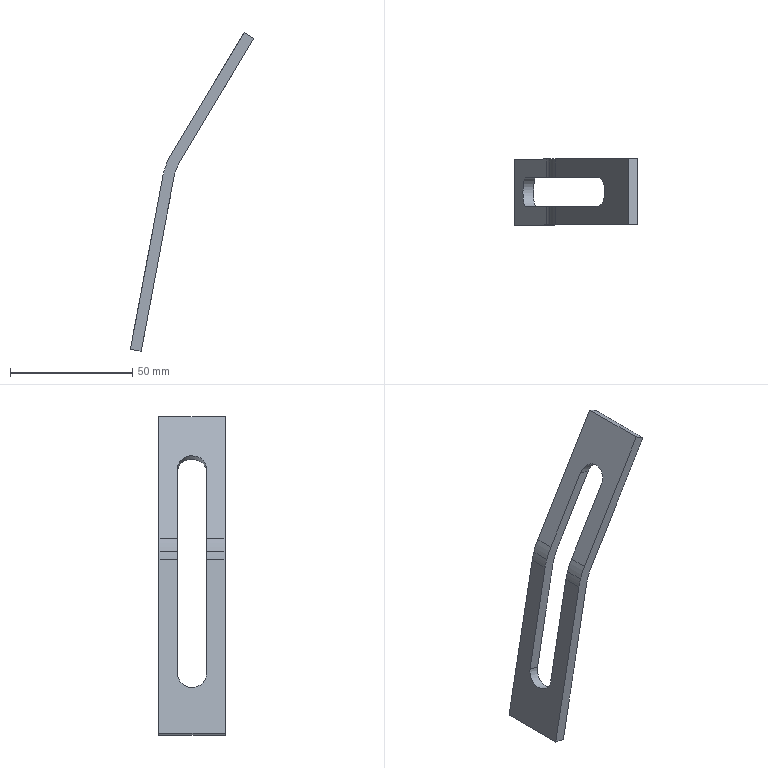Part | STEP file | 2026.6.15-Main Assembly图.sldasm-Part-201 | 1 solid | 20 faces | box 50.44 x 27 x 130.381 mm | volume 11515 mm3 | cylinder 10 | plane 10 | commonest cylinder face diameters 43.5 x4 52.5 x4 12 x2
STEP:
#1=CARTESIAN_POINT('',(-1667.232,1410.764,3344.403));
#2=VERTEX_POINT('',#1);
#3=CARTESIAN_POINT('',(-1667.232,1418.264,3344.403));
#4=VERTEX_POINT('',#3);
#5=CARTESIAN_POINT('',(-1667.232,1410.764,3344.403));
#6=DIRECTION('',(0.,1.,0.));
#7=VECTOR('',#6,1000.);
#8=LINE('',#5,#7);
#9=EDGE_CURVE('',#2,#4,#8,.T.);
#10=ORIENTED_EDGE('',*,*,#9,.F.);
#11=CARTESIAN_POINT('',(-1668.,1410.764,3341.468));
#12=VERTEX_POINT('',#11);
#13=CARTESIAN_POINT('',(-1646.625,1410.764,3337.444));
#14=DIRECTION('',(0.,1.,0.));
#15=DIRECTION('',(-0.9474,0.,0.3199));
#16=AXIS2_PLACEMENT_3D('',#13,#14,#15);
#17=CIRCLE('',#16,21.75);
#18=EDGE_CURVE('',#12,#2,#17,.T.);
#19=ORIENTED_EDGE('',*,*,#18,.F.);
#20=CARTESIAN_POINT('',(-1668.,1418.264,3341.468));
#21=VERTEX_POINT('',#20);
#22=CARTESIAN_POINT('',(-1668.,1410.764,3341.468));
#23=DIRECTION('',(0.,-1.,0.));
#24=VECTOR('',#23,1000.);
#25=LINE('',#22,#24);
#26=EDGE_CURVE('',#21,#12,#25,.T.);
#27=ORIENTED_EDGE('',*,*,#26,.F.);
#28=CARTESIAN_POINT('',(-1646.625,1418.264,3337.444));
#29=DIRECTION('',(0.,1.,0.));
#30=DIRECTION('',(-0.9474,0.,0.3199));
#31=AXIS2_PLACEMENT_3D('',#28,#29,#30);
#32=CIRCLE('',#31,21.75);
#33=EDGE_CURVE('',#21,#4,#32,.T.);
#34=ORIENTED_EDGE('',*,*,#33,.T.);
#35=EDGE_LOOP('',(#10,#19,#27,#34));
#36=FACE_OUTER_BOUND('',#35,.T.);
#37=CARTESIAN_POINT('',(-1646.625,1410.764,3337.444));
#38=DIRECTION('',(0.,1.,0.));
#39=DIRECTION('',(0.9474,0.,-0.3199));
#40=AXIS2_PLACEMENT_3D('',#37,#38,#39);
#41=CYLINDRICAL_SURFACE('',#40,21.75);
#42=ADVANCED_FACE('',(#36),#41,.F.);
#43=CARTESIAN_POINT('',(-1635.337,1410.764,3398.579));
#44=VERTEX_POINT('',#43);
#45=CARTESIAN_POINT('',(-1639.197,1410.764,3400.892));
#46=VERTEX_POINT('',#45);
#47=CARTESIAN_POINT('',(-1635.337,1410.764,3398.579));
#48=DIRECTION('',(-0.8577,0.,0.5141));
#49=VECTOR('',#48,1000.);
#50=LINE('',#47,#49);
#51=EDGE_CURVE('',#44,#46,#50,.T.);
#52=ORIENTED_EDGE('',*,*,#51,.F.);
#53=CARTESIAN_POINT('',(-1635.337,1437.764,3398.579));
#54=VERTEX_POINT('',#53);
#55=CARTESIAN_POINT('',(-1635.337,1410.764,3398.579));
#56=DIRECTION('',(0.,-1.,0.));
#57=VECTOR('',#56,1000.);
#58=LINE('',#55,#57);
#59=EDGE_CURVE('',#54,#44,#58,.T.);
#60=ORIENTED_EDGE('',*,*,#59,.F.);
#61=CARTESIAN_POINT('',(-1639.197,1437.764,3400.892));
#62=VERTEX_POINT('',#61);
#63=CARTESIAN_POINT('',(-1635.337,1437.764,3398.579));
#64=DIRECTION('',(-0.8577,0.,0.5141));
#65=VECTOR('',#64,1000.);
#66=LINE('',#63,#65);
#67=EDGE_CURVE('',#54,#62,#66,.T.);
#68=ORIENTED_EDGE('',*,*,#67,.T.);
#69=CARTESIAN_POINT('',(-1639.197,1410.764,3400.892));
#70=DIRECTION('',(0.,-1.,0.));
#71=VECTOR('',#70,1000.);
#72=LINE('',#69,#71);
#73=EDGE_CURVE('',#62,#46,#72,.T.);
#74=ORIENTED_EDGE('',*,*,#73,.T.);
#75=EDGE_LOOP('',(#52,#60,#68,#74));
#76=FACE_OUTER_BOUND('',#75,.T.);
#77=CARTESIAN_POINT('',(-1639.197,1410.764,3400.892));
#78=DIRECTION('',(0.5141,0.,0.8577));
#79=DIRECTION('',(-0.8577,0.,0.5141));
#80=AXIS2_PLACEMENT_3D('',#77,#78,#79);
#81=PLANE('',#80);
#82=ADVANCED_FACE('',(#76),#81,.T.);
#83=CARTESIAN_POINT('',(-1669.14,1430.264,3350.941));
#84=VERTEX_POINT('',#83);
#85=CARTESIAN_POINT('',(-1651.961,1430.264,3379.599));
#86=VERTEX_POINT('',#85);
#87=CARTESIAN_POINT('',(-1669.14,1430.264,3350.941));
#88=DIRECTION('',(0.5141,0.,0.8577));
#89=VECTOR('',#88,1000.);
#90=LINE('',#87,#89);
#91=EDGE_CURVE('',#84,#86,#90,.T.);
#92=ORIENTED_EDGE('',*,*,#91,.T.);
#93=CARTESIAN_POINT('',(-1651.961,1418.264,3379.599));
#94=VERTEX_POINT('',#93);
#95=CARTESIAN_POINT('',(-1651.961,1430.264,3379.599));
#96=CARTESIAN_POINT('',(-1645.647,1430.264,3390.132));
#97=CARTESIAN_POINT('',(-1645.647,1418.264,3390.132));
#98=CARTESIAN_POINT('',(-1651.961,1418.264,3379.599));
#99=(BOUNDED_CURVE()B_SPLINE_CURVE(3,(#95,#96,#97,#98),.UNSPECIFIED.,.F.,.F.)B_SPLINE_CURVE_WITH_KNOTS((4,4),(0.,1.),.UNSPECIFIED.)CURVE()GEOMETRIC_REPRESENTATION_ITEM()RATIONAL_B_SPLINE_CURVE((1.,0.3333,0.3333,1.))REPRESENTATION_ITEM(''));
#100=EDGE_CURVE('',#86,#94,#99,.T.);
#101=ORIENTED_EDGE('',*,*,#100,.T.);
#102=CARTESIAN_POINT('',(-1669.14,1418.264,3350.941));
#103=VERTEX_POINT('',#102);
#104=CARTESIAN_POINT('',(-1651.961,1418.264,3379.599));
#105=DIRECTION('',(-0.5141,0.,-0.8577));
#106=VECTOR('',#105,1000.);
#107=LINE('',#104,#106);
#108=EDGE_CURVE('',#94,#103,#107,.T.);
#109=ORIENTED_EDGE('',*,*,#108,.T.);
#110=CARTESIAN_POINT('',(-1669.14,1410.764,3350.941));
#111=VERTEX_POINT('',#110);
#112=CARTESIAN_POINT('',(-1669.14,1410.764,3350.941));
#113=DIRECTION('',(0.,1.,0.));
#114=VECTOR('',#113,1000.);
#115=LINE('',#112,#114);
#116=EDGE_CURVE('',#111,#103,#115,.T.);
#117=ORIENTED_EDGE('',*,*,#116,.F.);
#118=CARTESIAN_POINT('',(-1639.197,1410.764,3400.892));
#119=DIRECTION('',(-0.5141,0.,-0.8577));
#120=VECTOR('',#119,1000.);
#121=LINE('',#118,#120);
#122=EDGE_CURVE('',#46,#111,#121,.T.);
#123=ORIENTED_EDGE('',*,*,#122,.F.);
#124=ORIENTED_EDGE('',*,*,#73,.F.);
#125=CARTESIAN_POINT('',(-1669.14,1437.764,3350.941));
#126=VERTEX_POINT('',#125);
#127=CARTESIAN_POINT('',(-1639.197,1437.764,3400.892));
#128=DIRECTION('',(-0.5141,0.,-0.8577));
#129=VECTOR('',#128,1000.);
#130=LINE('',#127,#129);
#131=EDGE_CURVE('',#62,#126,#130,.T.);
#132=ORIENTED_EDGE('',*,*,#131,.T.);
#133=CARTESIAN_POINT('',(-1669.14,1410.764,3350.941));
#134=DIRECTION('',(0.,1.,0.));
#135=VECTOR('',#134,1000.);
#136=LINE('',#133,#135);
#137=EDGE_CURVE('',#84,#126,#136,.T.);
#138=ORIENTED_EDGE('',*,*,#137,.F.);
#139=EDGE_LOOP('',(#92,#101,#109,#117,#123,#124,#132,#138));
#140=FACE_OUTER_BOUND('',#139,.T.);
#141=CARTESIAN_POINT('',(-1639.197,1410.764,3400.892));
#142=DIRECTION('',(0.8577,0.,-0.5141));
#143=DIRECTION('',(0.,-1.,0.));
#144=AXIS2_PLACEMENT_3D('',#141,#142,#143);
#145=PLANE('',#144);
#146=ADVANCED_FACE('',(#140),#145,.F.);
#147=CARTESIAN_POINT('',(-1647.598,1418.264,3378.125));
#148=VERTEX_POINT('',#147);
#149=CARTESIAN_POINT('',(-1662.816,1418.264,3383.264));
#150=DIRECTION('',(-0.9474,0.,0.3199));
#151=VECTOR('',#150,1000.);
#152=LINE('',#149,#151);
#153=EDGE_CURVE('',#148,#94,#152,.T.);
#154=ORIENTED_EDGE('',*,*,#153,.T.);
#155=ORIENTED_EDGE('',*,*,#100,.F.);
#156=CARTESIAN_POINT('',(-1647.598,1430.264,3378.125));
#157=VERTEX_POINT('',#156);
#158=CARTESIAN_POINT('',(-1662.816,1430.264,3383.264));
#159=DIRECTION('',(0.9474,0.,-0.3199));
#160=VECTOR('',#159,1000.);
#161=LINE('',#158,#160);
#162=EDGE_CURVE('',#86,#157,#161,.T.);
#163=ORIENTED_EDGE('',*,*,#162,.T.);
#164=CARTESIAN_POINT('',(-1647.598,1418.264,3378.125));
#165=CARTESIAN_POINT('',(-1641.284,1418.264,3388.659));
#166=CARTESIAN_POINT('',(-1641.284,1430.264,3388.659));
#167=CARTESIAN_POINT('',(-1647.598,1430.264,3378.125));
#168=(BOUNDED_CURVE()B_SPLINE_CURVE(3,(#164,#165,#166,#167),.UNSPECIFIED.,.F.,.T.)B_SPLINE_CURVE_WITH_KNOTS((4,4),(0.,1.),.UNSPECIFIED.)CURVE()GEOMETRIC_REPRESENTATION_ITEM()RATIONAL_B_SPLINE_CURVE((1.,0.3333,0.3333,1.))REPRESENTATION_ITEM(''));
#169=EDGE_CURVE('',#148,#157,#168,.T.);
#170=ORIENTED_EDGE('',*,*,#169,.F.);
#171=EDGE_LOOP('',(#154,#155,#163,#170));
#172=FACE_OUTER_BOUND('',#171,.T.);
#173=CARTESIAN_POINT('',(-1662.816,1424.264,3383.264));
#174=DIRECTION('',(0.9474,0.,-0.3199));
#175=DIRECTION('',(0.,-1.,0.));
#176=AXIS2_PLACEMENT_3D('',#173,#174,#175);
#177=CYLINDRICAL_SURFACE('',#176,6.);
#178=ADVANCED_FACE('',(#172),#177,.F.);
#179=CARTESIAN_POINT('',(-1665.28,1418.264,3348.627));
#180=VERTEX_POINT('',#179);
#181=CARTESIAN_POINT('',(-1665.28,1418.264,3348.627));
#182=DIRECTION('',(0.5141,0.,0.8577));
#183=VECTOR('',#182,1000.);
#184=LINE('',#181,#183);
#185=EDGE_CURVE('',#180,#148,#184,.T.);
#186=ORIENTED_EDGE('',*,*,#185,.T.);
#187=ORIENTED_EDGE('',*,*,#169,.T.);
#188=CARTESIAN_POINT('',(-1665.28,1430.264,3348.627));
#189=VERTEX_POINT('',#188);
#190=CARTESIAN_POINT('',(-1647.598,1430.264,3378.125));
#191=DIRECTION('',(-0.5141,0.,-0.8577));
#192=VECTOR('',#191,1000.);
#193=LINE('',#190,#192);
#194=EDGE_CURVE('',#157,#189,#193,.T.);
#195=ORIENTED_EDGE('',*,*,#194,.T.);
#196=CARTESIAN_POINT('',(-1665.28,1437.764,3348.627));
#197=VERTEX_POINT('',#196);
#198=CARTESIAN_POINT('',(-1665.28,1410.764,3348.627));
#199=DIRECTION('',(0.,1.,0.));
#200=VECTOR('',#199,1000.);
#201=LINE('',#198,#200);
#202=EDGE_CURVE('',#189,#197,#201,.T.);
#203=ORIENTED_EDGE('',*,*,#202,.T.);
#204=CARTESIAN_POINT('',(-1665.28,1437.764,3348.627));
#205=DIRECTION('',(0.5141,0.,0.8577));
#206=VECTOR('',#205,1000.);
#207=LINE('',#204,#206);
#208=EDGE_CURVE('',#197,#54,#207,.T.);
#209=ORIENTED_EDGE('',*,*,#208,.T.);
#210=ORIENTED_EDGE('',*,*,#59,.T.);
#211=CARTESIAN_POINT('',(-1665.28,1410.764,3348.627));
#212=VERTEX_POINT('',#211);
#213=CARTESIAN_POINT('',(-1665.28,1410.764,3348.627));
#214=DIRECTION('',(0.5141,0.,0.8577));
#215=VECTOR('',#214,1000.);
#216=LINE('',#213,#215);
#217=EDGE_CURVE('',#212,#44,#216,.T.);
#218=ORIENTED_EDGE('',*,*,#217,.F.);
#219=CARTESIAN_POINT('',(-1665.28,1410.764,3348.627));
#220=DIRECTION('',(0.,1.,0.));
#221=VECTOR('',#220,1000.);
#222=LINE('',#219,#221);
#223=EDGE_CURVE('',#212,#180,#222,.T.);
#224=ORIENTED_EDGE('',*,*,#223,.T.);
#225=EDGE_LOOP('',(#186,#187,#195,#203,#209,#210,#218,#224));
#226=FACE_OUTER_BOUND('',#225,.T.);
#227=CARTESIAN_POINT('',(-1635.337,1410.764,3398.579));
#228=DIRECTION('',(0.8577,0.,-0.5141));
#229=DIRECTION('',(0.,-1.,0.));
#230=AXIS2_PLACEMENT_3D('',#227,#228,#229);
#231=PLANE('',#230);
#232=ADVANCED_FACE('',(#226),#231,.T.);
#233=CARTESIAN_POINT('',(-1667.232,1430.264,3344.403));
#234=VERTEX_POINT('',#233);
#235=CARTESIAN_POINT('',(-1667.232,1437.764,3344.403));
#236=VERTEX_POINT('',#235);
#237=CARTESIAN_POINT('',(-1667.232,1410.764,3344.403));
#238=DIRECTION('',(0.,1.,0.));
#239=VECTOR('',#238,1000.);
#240=LINE('',#237,#239);
#241=EDGE_CURVE('',#234,#236,#240,.T.);
#242=ORIENTED_EDGE('',*,*,#241,.F.);
#243=CARTESIAN_POINT('',(-1668.,1430.264,3341.468));
#244=VERTEX_POINT('',#243);
#245=CARTESIAN_POINT('',(-1646.625,1430.264,3337.444));
#246=DIRECTION('',(0.,-1.,0.));
#247=DIRECTION('',(-0.9474,0.,0.3199));
#248=AXIS2_PLACEMENT_3D('',#245,#246,#247);
#249=CIRCLE('',#248,21.75);
#250=EDGE_CURVE('',#234,#244,#249,.T.);
#251=ORIENTED_EDGE('',*,*,#250,.T.);
#252=CARTESIAN_POINT('',(-1668.,1437.764,3341.468));
#253=VERTEX_POINT('',#252);
#254=CARTESIAN_POINT('',(-1668.,1410.764,3341.468));
#255=DIRECTION('',(0.,-1.,0.));
#256=VECTOR('',#255,1000.);
#257=LINE('',#254,#256);
#258=EDGE_CURVE('',#253,#244,#257,.T.);
#259=ORIENTED_EDGE('',*,*,#258,.F.);
#260=CARTESIAN_POINT('',(-1646.625,1437.764,3337.444));
#261=DIRECTION('',(0.,1.,0.));
#262=DIRECTION('',(-0.9474,0.,0.3199));
#263=AXIS2_PLACEMENT_3D('',#260,#261,#262);
#264=CIRCLE('',#263,21.75);
#265=EDGE_CURVE('',#253,#236,#264,.T.);
#266=ORIENTED_EDGE('',*,*,#265,.T.);
#267=EDGE_LOOP('',(#242,#251,#259,#266));
#268=FACE_OUTER_BOUND('',#267,.T.);
#269=CARTESIAN_POINT('',(-1646.625,1410.764,3337.444));
#270=DIRECTION('',(0.,1.,0.));
#271=DIRECTION('',(0.9474,0.,-0.3199));
#272=AXIS2_PLACEMENT_3D('',#269,#270,#271);
#273=CYLINDRICAL_SURFACE('',#272,21.75);
#274=ADVANCED_FACE('',(#268),#273,.F.);
#275=CARTESIAN_POINT('',(-1681.355,1437.764,3270.511));
#276=VERTEX_POINT('',#275);
#277=CARTESIAN_POINT('',(-1681.355,1437.764,3270.511));
#278=DIRECTION('',(0.185,0.,0.9827));
#279=VECTOR('',#278,1000.);
#280=LINE('',#277,#279);
#281=EDGE_CURVE('',#276,#253,#280,.T.);
#282=ORIENTED_EDGE('',*,*,#281,.T.);
#283=ORIENTED_EDGE('',*,*,#258,.T.);
#284=CARTESIAN_POINT('',(-1676.824,1430.264,3294.585));
#285=VERTEX_POINT('',#284);
#286=CARTESIAN_POINT('',(-1668.,1430.264,3341.468));
#287=DIRECTION('',(-0.185,0.,-0.9827));
#288=VECTOR('',#287,1000.);
#289=LINE('',#286,#288);
#290=EDGE_CURVE('',#244,#285,#289,.T.);
#291=ORIENTED_EDGE('',*,*,#290,.T.);
#292=CARTESIAN_POINT('',(-1676.824,1418.264,3294.585));
#293=VERTEX_POINT('',#292);
#294=CARTESIAN_POINT('',(-1676.824,1430.264,3294.585));
#295=CARTESIAN_POINT('',(-1679.065,1430.264,3282.676));
#296=CARTESIAN_POINT('',(-1679.065,1418.264,3282.676));
#297=CARTESIAN_POINT('',(-1676.824,1418.264,3294.585));
#298=(BOUNDED_CURVE()B_SPLINE_CURVE(3,(#294,#295,#296,#297),.UNSPECIFIED.,.F.,.F.)B_SPLINE_CURVE_WITH_KNOTS((4,4),(0.,1.),.UNSPECIFIED.)CURVE()GEOMETRIC_REPRESENTATION_ITEM()RATIONAL_B_SPLINE_CURVE((1.,0.3333,0.3333,1.))REPRESENTATION_ITEM(''));
#299=EDGE_CURVE('',#285,#293,#298,.T.);
#300=ORIENTED_EDGE('',*,*,#299,.T.);
#301=CARTESIAN_POINT('',(-1676.824,1418.264,3294.585));
#302=DIRECTION('',(0.185,0.,0.9827));
#303=VECTOR('',#302,1000.);
#304=LINE('',#301,#303);
#305=EDGE_CURVE('',#293,#21,#304,.T.);
#306=ORIENTED_EDGE('',*,*,#305,.T.);
#307=ORIENTED_EDGE('',*,*,#26,.T.);
#308=CARTESIAN_POINT('',(-1681.355,1410.764,3270.511));
#309=VERTEX_POINT('',#308);
#310=CARTESIAN_POINT('',(-1681.355,1410.764,3270.511));
#311=DIRECTION('',(0.185,0.,0.9827));
#312=VECTOR('',#311,1000.);
#313=LINE('',#310,#312);
#314=EDGE_CURVE('',#309,#12,#313,.T.);
#315=ORIENTED_EDGE('',*,*,#314,.F.);
#316=CARTESIAN_POINT('',(-1681.355,1410.764,3270.511));
#317=DIRECTION('',(0.,-1.,0.));
#318=VECTOR('',#317,1000.);
#319=LINE('',#316,#318);
#320=EDGE_CURVE('',#276,#309,#319,.T.);
#321=ORIENTED_EDGE('',*,*,#320,.F.);
#322=EDGE_LOOP('',(#282,#283,#291,#300,#306,#307,#315,#321));
#323=FACE_OUTER_BOUND('',#322,.T.);
#324=CARTESIAN_POINT('',(-1668.,1410.764,3341.468));
#325=DIRECTION('',(0.9827,0.,-0.185));
#326=DIRECTION('',(0.,-1.,0.));
#327=AXIS2_PLACEMENT_3D('',#324,#325,#326);
#328=PLANE('',#327);
#329=ADVANCED_FACE('',(#323),#328,.T.);
#330=CARTESIAN_POINT('',(-1681.129,1418.264,3296.038));
#331=VERTEX_POINT('',#330);
#332=CARTESIAN_POINT('',(-1691.131,1418.264,3299.416));
#333=DIRECTION('',(-0.9474,0.,0.3199));
#334=VECTOR('',#333,1000.);
#335=LINE('',#332,#334);
#336=EDGE_CURVE('',#293,#331,#335,.T.);
#337=ORIENTED_EDGE('',*,*,#336,.T.);
#338=CARTESIAN_POINT('',(-1672.422,1418.264,3342.3));
#339=VERTEX_POINT('',#338);
#340=CARTESIAN_POINT('',(-1672.422,1418.264,3342.3));
#341=DIRECTION('',(0.185,0.,0.9827));
#342=VECTOR('',#341,1000.);
#343=LINE('',#340,#342);
#344=EDGE_CURVE('',#331,#339,#343,.T.);
#345=ORIENTED_EDGE('',*,*,#344,.T.);
#346=CARTESIAN_POINT('',(-1671.495,1418.264,3345.843));
#347=VERTEX_POINT('',#346);
#348=CARTESIAN_POINT('',(-1646.625,1418.264,3337.444));
#349=DIRECTION('',(0.,-1.,0.));
#350=DIRECTION('',(-0.9474,0.,0.3199));
#351=AXIS2_PLACEMENT_3D('',#348,#349,#350);
#352=CIRCLE('',#351,26.25);
#353=EDGE_CURVE('',#347,#339,#352,.T.);
#354=ORIENTED_EDGE('',*,*,#353,.F.);
#355=CARTESIAN_POINT('',(-1646.625,1418.264,3337.444));
#356=DIRECTION('',(0.,-1.,0.));
#357=DIRECTION('',(-0.9474,0.,0.3199));
#358=AXIS2_PLACEMENT_3D('',#355,#356,#357);
#359=CIRCLE('',#358,26.25);
#360=EDGE_CURVE('',#103,#347,#359,.T.);
#361=ORIENTED_EDGE('',*,*,#360,.F.);
#362=ORIENTED_EDGE('',*,*,#108,.F.);
#363=ORIENTED_EDGE('',*,*,#153,.F.);
#364=ORIENTED_EDGE('',*,*,#185,.F.);
#365=CARTESIAN_POINT('',(-1646.625,1418.264,3337.444));
#366=DIRECTION('',(0.,1.,0.));
#367=DIRECTION('',(-0.9474,0.,0.3199));
#368=AXIS2_PLACEMENT_3D('',#365,#366,#367);
#369=CIRCLE('',#368,21.75);
#370=EDGE_CURVE('',#4,#180,#369,.T.);
#371=ORIENTED_EDGE('',*,*,#370,.F.);
#372=ORIENTED_EDGE('',*,*,#33,.F.);
#373=ORIENTED_EDGE('',*,*,#305,.F.);
#374=EDGE_LOOP('',(#337,#345,#354,#361,#362,#363,#364,#371,#372,#373));
#375=FACE_OUTER_BOUND('',#374,.T.);
#376=CARTESIAN_POINT('',(-1662.816,1418.264,3383.264));
#377=DIRECTION('',(0.,-1.,0.));
#378=DIRECTION('',(-1.,0.,0.));
#379=AXIS2_PLACEMENT_3D('',#376,#377,#378);
#380=PLANE('',#379);
#381=ADVANCED_FACE('',(#375),#380,.F.);
#382=CARTESIAN_POINT('',(-1671.495,1410.764,3345.843));
#383=VERTEX_POINT('',#382);
#384=CARTESIAN_POINT('',(-1671.495,1410.764,3345.843));
#385=DIRECTION('',(0.,1.,0.));
#386=VECTOR('',#385,1000.);
#387=LINE('',#384,#386);
#388=EDGE_CURVE('',#383,#347,#387,.T.);
#389=ORIENTED_EDGE('',*,*,#388,.F.);
#390=CARTESIAN_POINT('',(-1646.625,1410.764,3337.444));
#391=DIRECTION('',(0.,-1.,0.));
#392=DIRECTION('',(-0.9474,0.,0.3199));
#393=AXIS2_PLACEMENT_3D('',#390,#391,#392);
#394=CIRCLE('',#393,26.25);
#395=EDGE_CURVE('',#111,#383,#394,.T.);
#396=ORIENTED_EDGE('',*,*,#395,.F.);
#397=ORIENTED_EDGE('',*,*,#116,.T.);
#398=ORIENTED_EDGE('',*,*,#360,.T.);
#399=EDGE_LOOP('',(#389,#396,#397,#398));
#400=FACE_OUTER_BOUND('',#399,.T.);
#401=CARTESIAN_POINT('',(-1646.625,1410.764,3337.444));
#402=DIRECTION('',(0.,1.,0.));
#403=DIRECTION('',(0.9474,0.,-0.3199));
#404=AXIS2_PLACEMENT_3D('',#401,#402,#403);
#405=CYLINDRICAL_SURFACE('',#404,26.25);
#406=ADVANCED_FACE('',(#400),#405,.T.);
#407=ORIENTED_EDGE('',*,*,#122,.T.);
#408=ORIENTED_EDGE('',*,*,#395,.T.);
#409=CARTESIAN_POINT('',(-1672.422,1410.764,3342.3));
#410=VERTEX_POINT('',#409);
#411=CARTESIAN_POINT('',(-1646.625,1410.764,3337.444));
#412=DIRECTION('',(0.,-1.,0.));
#413=DIRECTION('',(-0.9474,0.,0.3199));
#414=AXIS2_PLACEMENT_3D('',#411,#412,#413);
#415=CIRCLE('',#414,26.25);
#416=EDGE_CURVE('',#383,#410,#415,.T.);
#417=ORIENTED_EDGE('',*,*,#416,.T.);
#418=CARTESIAN_POINT('',(-1685.777,1410.764,3271.343));
#419=VERTEX_POINT('',#418);
#420=CARTESIAN_POINT('',(-1672.422,1410.764,3342.3));
#421=DIRECTION('',(-0.185,0.,-0.9827));
#422=VECTOR('',#421,1000.);
#423=LINE('',#420,#422);
#424=EDGE_CURVE('',#410,#419,#423,.T.);
#425=ORIENTED_EDGE('',*,*,#424,.T.);
#426=CARTESIAN_POINT('',(-1681.355,1410.764,3270.511));
#427=DIRECTION('',(-0.9827,0.,0.185));
#428=VECTOR('',#427,1000.);
#429=LINE('',#426,#428);
#430=EDGE_CURVE('',#309,#419,#429,.T.);
#431=ORIENTED_EDGE('',*,*,#430,.F.);
#432=ORIENTED_EDGE('',*,*,#314,.T.);
#433=ORIENTED_EDGE('',*,*,#18,.T.);
#434=CARTESIAN_POINT('',(-1646.625,1410.764,3337.444));
#435=DIRECTION('',(0.,1.,0.));
#436=DIRECTION('',(-0.9474,0.,0.3199));
#437=AXIS2_PLACEMENT_3D('',#434,#435,#436);
#438=CIRCLE('',#437,21.75);
#439=EDGE_CURVE('',#2,#212,#438,.T.);
#440=ORIENTED_EDGE('',*,*,#439,.T.);
#441=ORIENTED_EDGE('',*,*,#217,.T.);
#442=ORIENTED_EDGE('',*,*,#51,.T.);
#443=EDGE_LOOP('',(#407,#408,#417,#425,#431,#432,#433,#440,#441,#442));
#444=FACE_OUTER_BOUND('',#443,.T.);
#445=CARTESIAN_POINT('',(-1646.625,1410.764,3337.444));
#446=DIRECTION('',(0.,-1.,0.));
#447=DIRECTION('',(0.,0.,-1.));
#448=AXIS2_PLACEMENT_3D('',#445,#446,#447);
#449=PLANE('',#448);
#450=ADVANCED_FACE('',(#444),#449,.T.);
#451=ORIENTED_EDGE('',*,*,#430,.T.);
#452=CARTESIAN_POINT('',(-1685.777,1437.764,3271.343));
#453=VERTEX_POINT('',#452);
#454=CARTESIAN_POINT('',(-1685.777,1410.764,3271.343));
#455=DIRECTION('',(0.,1.,0.));
#456=VECTOR('',#455,1000.);
#457=LINE('',#454,#456);
#458=EDGE_CURVE('',#419,#453,#457,.T.);
#459=ORIENTED_EDGE('',*,*,#458,.T.);
#460=CARTESIAN_POINT('',(-1685.777,1437.764,3271.343));
#461=DIRECTION('',(0.9827,0.,-0.185));
#462=VECTOR('',#461,1000.);
#463=LINE('',#460,#462);
#464=EDGE_CURVE('',#453,#276,#463,.T.);
#465=ORIENTED_EDGE('',*,*,#464,.T.);
#466=ORIENTED_EDGE('',*,*,#320,.T.);
#467=EDGE_LOOP('',(#451,#459,#465,#466));
#468=FACE_OUTER_BOUND('',#467,.T.);
#469=CARTESIAN_POINT('',(-1681.355,1410.764,3270.511));
#470=DIRECTION('',(-0.185,0.,-0.9827));
#471=DIRECTION('',(0.,1.,0.));
#472=AXIS2_PLACEMENT_3D('',#469,#470,#471);
#473=PLANE('',#472);
#474=ADVANCED_FACE('',(#468),#473,.T.);
#475=CARTESIAN_POINT('',(-1671.495,1437.764,3345.843));
#476=VERTEX_POINT('',#475);
#477=CARTESIAN_POINT('',(-1646.625,1437.764,3337.444));
#478=DIRECTION('',(0.,-1.,0.));
#479=DIRECTION('',(-0.9474,0.,0.3199));
#480=AXIS2_PLACEMENT_3D('',#477,#478,#479);
#481=CIRCLE('',#480,26.25);
#482=EDGE_CURVE('',#126,#476,#481,.T.);
#483=ORIENTED_EDGE('',*,*,#482,.F.);
#484=ORIENTED_EDGE('',*,*,#131,.F.);
#485=ORIENTED_EDGE('',*,*,#67,.F.);
#486=ORIENTED_EDGE('',*,*,#208,.F.);
#487=CARTESIAN_POINT('',(-1646.625,1437.764,3337.444));
#488=DIRECTION('',(0.,1.,0.));
#489=DIRECTION('',(-0.9474,0.,0.3199));
#490=AXIS2_PLACEMENT_3D('',#487,#488,#489);
#491=CIRCLE('',#490,21.75);
#492=EDGE_CURVE('',#236,#197,#491,.T.);
#493=ORIENTED_EDGE('',*,*,#492,.F.);
#494=ORIENTED_EDGE('',*,*,#265,.F.);
#495=ORIENTED_EDGE('',*,*,#281,.F.);
#496=ORIENTED_EDGE('',*,*,#464,.F.);
#497=CARTESIAN_POINT('',(-1672.422,1437.764,3342.3));
#498=VERTEX_POINT('',#497);
#499=CARTESIAN_POINT('',(-1672.422,1437.764,3342.3));
#500=DIRECTION('',(0.185,0.,0.9827));
#501=VECTOR('',#500,1000.);
#502=LINE('',#499,#501);
#503=EDGE_CURVE('',#453,#498,#502,.T.);
#504=ORIENTED_EDGE('',*,*,#503,.T.);
#505=CARTESIAN_POINT('',(-1646.625,1437.764,3337.444));
#506=DIRECTION('',(0.,-1.,0.));
#507=DIRECTION('',(-0.9474,0.,0.3199));
#508=AXIS2_PLACEMENT_3D('',#505,#506,#507);
#509=CIRCLE('',#508,26.25);
#510=EDGE_CURVE('',#476,#498,#509,.T.);
#511=ORIENTED_EDGE('',*,*,#510,.F.);
#512=EDGE_LOOP('',(#483,#484,#485,#486,#493,#494,#495,#496,#504,#511));
#513=FACE_OUTER_BOUND('',#512,.T.);
#514=CARTESIAN_POINT('',(-1646.625,1437.764,3337.444));
#515=DIRECTION('',(0.,-1.,0.));
#516=DIRECTION('',(0.,0.,-1.));
#517=AXIS2_PLACEMENT_3D('',#514,#515,#516);
#518=PLANE('',#517);
#519=ADVANCED_FACE('',(#513),#518,.F.);
#520=CARTESIAN_POINT('',(-1671.495,1430.264,3345.843));
#521=VERTEX_POINT('',#520);
#522=CARTESIAN_POINT('',(-1671.495,1410.764,3345.843));
#523=DIRECTION('',(0.,1.,0.));
#524=VECTOR('',#523,1000.);
#525=LINE('',#522,#524);
#526=EDGE_CURVE('',#521,#476,#525,.T.);
#527=ORIENTED_EDGE('',*,*,#526,.F.);
#528=CARTESIAN_POINT('',(-1646.625,1430.264,3337.444));
#529=DIRECTION('',(0.,1.,0.));
#530=DIRECTION('',(-0.9474,0.,0.3199));
#531=AXIS2_PLACEMENT_3D('',#528,#529,#530);
#532=CIRCLE('',#531,26.25);
#533=EDGE_CURVE('',#521,#84,#532,.T.);
#534=ORIENTED_EDGE('',*,*,#533,.T.);
#535=ORIENTED_EDGE('',*,*,#137,.T.);
#536=ORIENTED_EDGE('',*,*,#482,.T.);
#537=EDGE_LOOP('',(#527,#534,#535,#536));
#538=FACE_OUTER_BOUND('',#537,.T.);
#539=CARTESIAN_POINT('',(-1646.625,1410.764,3337.444));
#540=DIRECTION('',(0.,1.,0.));
#541=DIRECTION('',(0.9474,0.,-0.3199));
#542=AXIS2_PLACEMENT_3D('',#539,#540,#541);
#543=CYLINDRICAL_SURFACE('',#542,26.25);
#544=ADVANCED_FACE('',(#538),#543,.T.);
#545=CARTESIAN_POINT('',(-1646.625,1430.264,3337.444));
#546=DIRECTION('',(0.,-1.,0.));
#547=DIRECTION('',(-0.9474,0.,0.3199));
#548=AXIS2_PLACEMENT_3D('',#545,#546,#547);
#549=CIRCLE('',#548,21.75);
#550=EDGE_CURVE('',#189,#234,#549,.T.);
#551=ORIENTED_EDGE('',*,*,#550,.F.);
#552=ORIENTED_EDGE('',*,*,#194,.F.);
#553=ORIENTED_EDGE('',*,*,#162,.F.);
#554=ORIENTED_EDGE('',*,*,#91,.F.);
#555=ORIENTED_EDGE('',*,*,#533,.F.);
#556=CARTESIAN_POINT('',(-1672.422,1430.264,3342.3));
#557=VERTEX_POINT('',#556);
#558=CARTESIAN_POINT('',(-1646.625,1430.264,3337.444));
#559=DIRECTION('',(0.,1.,0.));
#560=DIRECTION('',(-0.9474,0.,0.3199));
#561=AXIS2_PLACEMENT_3D('',#558,#559,#560);
#562=CIRCLE('',#561,26.25);
#563=EDGE_CURVE('',#557,#521,#562,.T.);
#564=ORIENTED_EDGE('',*,*,#563,.F.);
#565=CARTESIAN_POINT('',(-1681.129,1430.264,3296.038));
#566=VERTEX_POINT('',#565);
#567=CARTESIAN_POINT('',(-1672.422,1430.264,3342.3));
#568=DIRECTION('',(-0.185,0.,-0.9827));
#569=VECTOR('',#568,1000.);
#570=LINE('',#567,#569);
#571=EDGE_CURVE('',#557,#566,#570,.T.);
#572=ORIENTED_EDGE('',*,*,#571,.T.);
#573=CARTESIAN_POINT('',(-1691.131,1430.264,3299.416));
#574=DIRECTION('',(0.9474,0.,-0.3199));
#575=VECTOR('',#574,1000.);
#576=LINE('',#573,#575);
#577=EDGE_CURVE('',#566,#285,#576,.T.);
#578=ORIENTED_EDGE('',*,*,#577,.T.);
#579=ORIENTED_EDGE('',*,*,#290,.F.);
#580=ORIENTED_EDGE('',*,*,#250,.F.);
#581=EDGE_LOOP('',(#551,#552,#553,#554,#555,#564,#572,#578,#579,#580));
#582=FACE_OUTER_BOUND('',#581,.T.);
#583=CARTESIAN_POINT('',(-1662.816,1430.264,3383.264));
#584=DIRECTION('',(0.,1.,0.));
#585=DIRECTION('',(0.,0.,-1.));
#586=AXIS2_PLACEMENT_3D('',#583,#584,#585);
#587=PLANE('',#586);
#588=ADVANCED_FACE('',(#582),#587,.F.);
#589=ORIENTED_EDGE('',*,*,#299,.F.);
#590=ORIENTED_EDGE('',*,*,#577,.F.);
#591=CARTESIAN_POINT('',(-1681.129,1430.264,3296.038));
#592=CARTESIAN_POINT('',(-1683.371,1430.264,3284.13));
#593=CARTESIAN_POINT('',(-1683.371,1418.264,3284.13));
#594=CARTESIAN_POINT('',(-1681.129,1418.264,3296.038));
#595=(BOUNDED_CURVE()B_SPLINE_CURVE(3,(#591,#592,#593,#594),.UNSPECIFIED.,.F.,.F.)B_SPLINE_CURVE_WITH_KNOTS((4,4),(0.,1.),.UNSPECIFIED.)CURVE()GEOMETRIC_REPRESENTATION_ITEM()RATIONAL_B_SPLINE_CURVE((1.,0.3333,0.3333,1.))REPRESENTATION_ITEM(''));
#596=EDGE_CURVE('',#566,#331,#595,.T.);
#597=ORIENTED_EDGE('',*,*,#596,.T.);
#598=ORIENTED_EDGE('',*,*,#336,.F.);
#599=EDGE_LOOP('',(#589,#590,#597,#598));
#600=FACE_OUTER_BOUND('',#599,.T.);
#601=CARTESIAN_POINT('',(-1691.131,1424.264,3299.416));
#602=DIRECTION('',(0.9474,0.,-0.3199));
#603=DIRECTION('',(0.,-1.,0.));
#604=AXIS2_PLACEMENT_3D('',#601,#602,#603);
#605=CYLINDRICAL_SURFACE('',#604,6.);
#606=ADVANCED_FACE('',(#600),#605,.F.);
#607=ORIENTED_EDGE('',*,*,#571,.F.);
#608=CARTESIAN_POINT('',(-1672.422,1410.764,3342.3));
#609=DIRECTION('',(0.,-1.,0.));
#610=VECTOR('',#609,1000.);
#611=LINE('',#608,#610);
#612=EDGE_CURVE('',#498,#557,#611,.T.);
#613=ORIENTED_EDGE('',*,*,#612,.F.);
#614=ORIENTED_EDGE('',*,*,#503,.F.);
#615=ORIENTED_EDGE('',*,*,#458,.F.);
#616=ORIENTED_EDGE('',*,*,#424,.F.);
#617=CARTESIAN_POINT('',(-1672.422,1410.764,3342.3));
#618=DIRECTION('',(0.,-1.,0.));
#619=VECTOR('',#618,1000.);
#620=LINE('',#617,#619);
#621=EDGE_CURVE('',#339,#410,#620,.T.);
#622=ORIENTED_EDGE('',*,*,#621,.F.);
#623=ORIENTED_EDGE('',*,*,#344,.F.);
#624=ORIENTED_EDGE('',*,*,#596,.F.);
#625=EDGE_LOOP('',(#607,#613,#614,#615,#616,#622,#623,#624));
#626=FACE_OUTER_BOUND('',#625,.T.);
#627=CARTESIAN_POINT('',(-1672.422,1410.764,3342.3));
#628=DIRECTION('',(0.9827,0.,-0.185));
#629=DIRECTION('',(0.,-1.,0.));
#630=AXIS2_PLACEMENT_3D('',#627,#628,#629);
#631=PLANE('',#630);
#632=ADVANCED_FACE('',(#626),#631,.F.);
#633=ORIENTED_EDGE('',*,*,#439,.F.);
#634=ORIENTED_EDGE('',*,*,#9,.T.);
#635=ORIENTED_EDGE('',*,*,#370,.T.);
#636=ORIENTED_EDGE('',*,*,#223,.F.);
#637=EDGE_LOOP('',(#633,#634,#635,#636));
#638=FACE_OUTER_BOUND('',#637,.T.);
#639=CARTESIAN_POINT('',(-1646.625,1410.764,3337.444));
#640=DIRECTION('',(0.,1.,0.));
#641=DIRECTION('',(0.9474,0.,-0.3199));
#642=AXIS2_PLACEMENT_3D('',#639,#640,#641);
#643=CYLINDRICAL_SURFACE('',#642,21.75);
#644=ADVANCED_FACE('',(#638),#643,.F.);
#645=ORIENTED_EDGE('',*,*,#550,.T.);
#646=ORIENTED_EDGE('',*,*,#241,.T.);
#647=ORIENTED_EDGE('',*,*,#492,.T.);
#648=ORIENTED_EDGE('',*,*,#202,.F.);
#649=EDGE_LOOP('',(#645,#646,#647,#648));
#650=FACE_OUTER_BOUND('',#649,.T.);
#651=CARTESIAN_POINT('',(-1646.625,1410.764,3337.444));
#652=DIRECTION('',(0.,1.,0.));
#653=DIRECTION('',(0.9474,0.,-0.3199));
#654=AXIS2_PLACEMENT_3D('',#651,#652,#653);
#655=CYLINDRICAL_SURFACE('',#654,21.75);
#656=ADVANCED_FACE('',(#650),#655,.F.);
#657=ORIENTED_EDGE('',*,*,#416,.F.);
#658=ORIENTED_EDGE('',*,*,#388,.T.);
#659=ORIENTED_EDGE('',*,*,#353,.T.);
#660=ORIENTED_EDGE('',*,*,#621,.T.);
#661=EDGE_LOOP('',(#657,#658,#659,#660));
#662=FACE_OUTER_BOUND('',#661,.T.);
#663=CARTESIAN_POINT('',(-1646.625,1410.764,3337.444));
#664=DIRECTION('',(0.,1.,0.));
#665=DIRECTION('',(0.9474,0.,-0.3199));
#666=AXIS2_PLACEMENT_3D('',#663,#664,#665);
#667=CYLINDRICAL_SURFACE('',#666,26.25);
#668=ADVANCED_FACE('',(#662),#667,.T.);
#669=ORIENTED_EDGE('',*,*,#563,.T.);
#670=ORIENTED_EDGE('',*,*,#526,.T.);
#671=ORIENTED_EDGE('',*,*,#510,.T.);
#672=ORIENTED_EDGE('',*,*,#612,.T.);
#673=EDGE_LOOP('',(#669,#670,#671,#672));
#674=FACE_OUTER_BOUND('',#673,.T.);
#675=CARTESIAN_POINT('',(-1646.625,1410.764,3337.444));
#676=DIRECTION('',(0.,1.,0.));
#677=DIRECTION('',(0.9474,0.,-0.3199));
#678=AXIS2_PLACEMENT_3D('',#675,#676,#677);
#679=CYLINDRICAL_SURFACE('',#678,26.25);
#680=ADVANCED_FACE('',(#674),#679,.T.);
#681=CLOSED_SHELL('',(#42,#82,#146,#178,#232,#274,#329,#381,#406,#450,#474,#519,#544,#588,#606,#632,#644,#656,#668,#680));
#682=MANIFOLD_SOLID_BREP('',#681);
#683=CARTESIAN_POINT('',(0.,0.,0.));
#684=DIRECTION('',(0.,0.,1.));
#685=DIRECTION('',(1.,0.,0.));
#686=AXIS2_PLACEMENT_3D('',#683,#684,#685);
#687=(LENGTH_UNIT()NAMED_UNIT(*)SI_UNIT(.MILLI.,.METRE.));
#688=UNCERTAINTY_MEASURE_WITH_UNIT(LENGTH_MEASURE(0.00001),#687,'','');
#689=(NAMED_UNIT(*)PLANE_ANGLE_UNIT()SI_UNIT($,.RADIAN.));
#690=(NAMED_UNIT(*)SI_UNIT($,.STERADIAN.)SOLID_ANGLE_UNIT());
#691=(GEOMETRIC_REPRESENTATION_CONTEXT(3)GLOBAL_UNCERTAINTY_ASSIGNED_CONTEXT((#688))GLOBAL_UNIT_ASSIGNED_CONTEXT((#687,#689,#690))REPRESENTATION_CONTEXT('',''));
#692=ADVANCED_BREP_SHAPE_REPRESENTATION('',(#682,#686),#691);